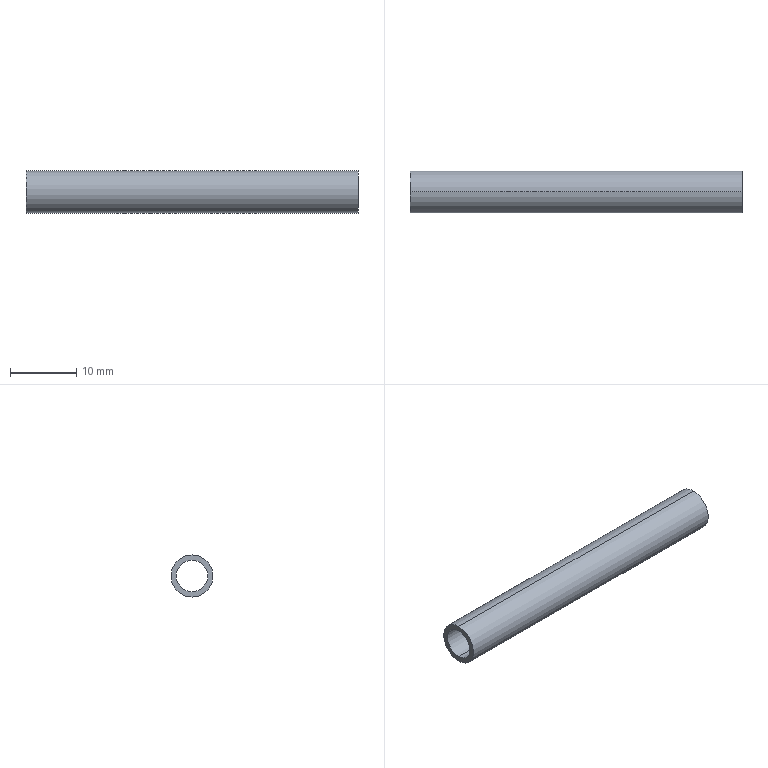Part | STEP file | copper tube 28_default_machined_ | 1 solid | 6 faces | box 50 x 6.35 x 6.35 mm | volume 697.434 mm3 | cylinder 4 | plane 2 | commonest cylinder face diameters 4.75 x2 6.35 x2
STEP:
#1=CARTESIAN_POINT('',(0.,0.,0.));
#2=DIRECTION('',(0.,0.,1.));
#3=DIRECTION('',(1.,0.,0.));
#4=AXIS2_PLACEMENT_3D('',#1,#2,#3);
#5=CARTESIAN_POINT('',(-50.,0.,-3.175));
#6=VERTEX_POINT('',#5);
#7=CARTESIAN_POINT('',(-50.,0.,3.175));
#8=VERTEX_POINT('',#7);
#9=CARTESIAN_POINT('',(-50.,0.,0.));
#10=DIRECTION('',(1.,0.,0.));
#11=DIRECTION('',(0.,0.,-1.));
#12=AXIS2_PLACEMENT_3D('',#9,#10,#11);
#13=CIRCLE('',#12,3.175);
#14=CARTESIAN_POINT('',(-50.,0.,0.));
#15=DIRECTION('',(1.,0.,0.));
#16=DIRECTION('',(0.,0.,-1.));
#17=AXIS2_PLACEMENT_3D('',#14,#15,#16);
#18=CYLINDRICAL_SURFACE('',#17,3.175);
#19=CARTESIAN_POINT('',(0.,0.));
#20=DIRECTION('',(1.,0.));
#21=VECTOR('',#20,1.);
#22=LINE('',#19,#21);
#23=(GEOMETRIC_REPRESENTATION_CONTEXT(2)PARAMETRIC_REPRESENTATION_CONTEXT()REPRESENTATION_CONTEXT('',''));
#24=DEFINITIONAL_REPRESENTATION('',(#22),#23);
#25=PCURVE('',#18,#24);
#26=CARTESIAN_POINT('',(-50.,0.,0.));
#27=DIRECTION('',(-1.,0.,0.));
#28=DIRECTION('',(0.,0.,1.));
#29=AXIS2_PLACEMENT_3D('',#26,#27,#28);
#30=PLANE('',#29);
#31=CARTESIAN_POINT('',(-3.175,0.));
#32=CARTESIAN_POINT('',(-3.175,5.499));
#33=CARTESIAN_POINT('',(1.587,2.75));
#34=CARTESIAN_POINT('',(6.35,0.));
#35=CARTESIAN_POINT('',(1.587,-2.75));
#36=CARTESIAN_POINT('',(-3.175,-5.499));
#37=CARTESIAN_POINT('',(-3.175,0.));
#38=(BOUNDED_CURVE()B_SPLINE_CURVE(2,(#31,#32,#33,#34,#35,#36,#37),.UNSPECIFIED.,.T.,.F.)B_SPLINE_CURVE_WITH_KNOTS((1,2,2,2,2,1),(-2.094,0.,2.094,4.189,6.283,8.378),.UNSPECIFIED.)CURVE()GEOMETRIC_REPRESENTATION_ITEM()RATIONAL_B_SPLINE_CURVE((1.,0.5,1.,0.5,1.,0.5,1.))REPRESENTATION_ITEM(''));
#39=(GEOMETRIC_REPRESENTATION_CONTEXT(2)PARAMETRIC_REPRESENTATION_CONTEXT()REPRESENTATION_CONTEXT('',''));
#40=DEFINITIONAL_REPRESENTATION('',(#38),#39);
#41=PCURVE('',#30,#40);
#42=SURFACE_CURVE('',#13,(#25,#41),.PCURVE_S1.);
#43=EDGE_CURVE('',#6,#8,#42,.T.);
#44=ORIENTED_EDGE('',*,*,#43,.T.);
#45=CARTESIAN_POINT('',(0.,0.,3.175));
#46=VERTEX_POINT('',#45);
#47=CARTESIAN_POINT('',(-50.,0.,3.175));
#48=DIRECTION('',(1.,0.,0.));
#49=VECTOR('',#48,1.);
#50=LINE('',#47,#49);
#51=CARTESIAN_POINT('',(3.142,0.));
#52=DIRECTION('',(0.,1.));
#53=VECTOR('',#52,1.);
#54=LINE('',#51,#53);
#55=(GEOMETRIC_REPRESENTATION_CONTEXT(2)PARAMETRIC_REPRESENTATION_CONTEXT()REPRESENTATION_CONTEXT('',''));
#56=DEFINITIONAL_REPRESENTATION('',(#54),#55);
#57=PCURVE('',#18,#56);
#58=CARTESIAN_POINT('',(-50.,0.,0.));
#59=DIRECTION('',(1.,0.,0.));
#60=DIRECTION('',(0.,0.,-1.));
#61=AXIS2_PLACEMENT_3D('',#58,#59,#60);
#62=CYLINDRICAL_SURFACE('',#61,3.175);
#63=CARTESIAN_POINT('',(3.142,0.));
#64=DIRECTION('',(0.,1.));
#65=VECTOR('',#64,1.);
#66=LINE('',#63,#65);
#67=(GEOMETRIC_REPRESENTATION_CONTEXT(2)PARAMETRIC_REPRESENTATION_CONTEXT()REPRESENTATION_CONTEXT('',''));
#68=DEFINITIONAL_REPRESENTATION('',(#66),#67);
#69=PCURVE('',#62,#68);
#70=SURFACE_CURVE('',#50,(#57,#69),.PCURVE_S1.);
#71=EDGE_CURVE('',#8,#46,#70,.T.);
#72=ORIENTED_EDGE('',*,*,#71,.T.);
#73=CARTESIAN_POINT('',(0.,0.,-3.175));
#74=VERTEX_POINT('',#73);
#75=CARTESIAN_POINT('',(0.,0.,0.));
#76=DIRECTION('',(-1.,0.,0.));
#77=DIRECTION('',(0.,0.,-1.));
#78=AXIS2_PLACEMENT_3D('',#75,#76,#77);
#79=CIRCLE('',#78,3.175);
#80=CARTESIAN_POINT('',(6.283,50.));
#81=DIRECTION('',(-1.,0.));
#82=VECTOR('',#81,1.);
#83=LINE('',#80,#82);
#84=(GEOMETRIC_REPRESENTATION_CONTEXT(2)PARAMETRIC_REPRESENTATION_CONTEXT()REPRESENTATION_CONTEXT('',''));
#85=DEFINITIONAL_REPRESENTATION('',(#83),#84);
#86=PCURVE('',#18,#85);
#87=CARTESIAN_POINT('',(0.,0.,0.));
#88=DIRECTION('',(-1.,0.,0.));
#89=DIRECTION('',(0.,0.,1.));
#90=AXIS2_PLACEMENT_3D('',#87,#88,#89);
#91=PLANE('',#90);
#92=CARTESIAN_POINT('',(0.,0.));
#93=DIRECTION('',(-1.,0.));
#94=AXIS2_PLACEMENT_2D('',#92,#93);
#95=CIRCLE('',#94,3.175);
#96=(GEOMETRIC_REPRESENTATION_CONTEXT(2)PARAMETRIC_REPRESENTATION_CONTEXT()REPRESENTATION_CONTEXT('',''));
#97=DEFINITIONAL_REPRESENTATION('',(#95),#96);
#98=PCURVE('',#91,#97);
#99=SURFACE_CURVE('',#79,(#86,#98),.PCURVE_S1.);
#100=EDGE_CURVE('',#46,#74,#99,.T.);
#101=ORIENTED_EDGE('',*,*,#100,.T.);
#102=CARTESIAN_POINT('',(-50.,0.,-3.175));
#103=DIRECTION('',(1.,0.,0.));
#104=VECTOR('',#103,1.);
#105=LINE('',#102,#104);
#106=CARTESIAN_POINT('',(0.,0.));
#107=DIRECTION('',(0.,1.));
#108=VECTOR('',#107,1.);
#109=LINE('',#106,#108);
#110=(GEOMETRIC_REPRESENTATION_CONTEXT(2)PARAMETRIC_REPRESENTATION_CONTEXT()REPRESENTATION_CONTEXT('',''));
#111=DEFINITIONAL_REPRESENTATION('',(#109),#110);
#112=PCURVE('',#18,#111);
#113=CARTESIAN_POINT('',(6.283,0.));
#114=DIRECTION('',(0.,1.));
#115=VECTOR('',#114,1.);
#116=LINE('',#113,#115);
#117=(GEOMETRIC_REPRESENTATION_CONTEXT(2)PARAMETRIC_REPRESENTATION_CONTEXT()REPRESENTATION_CONTEXT('',''));
#118=DEFINITIONAL_REPRESENTATION('',(#116),#117);
#119=PCURVE('',#62,#118);
#120=SURFACE_CURVE('',#105,(#112,#119),.PCURVE_S1.);
#121=EDGE_CURVE('',#6,#74,#120,.T.);
#122=ORIENTED_EDGE('',*,*,#121,.F.);
#123=EDGE_LOOP('',(#44,#72,#101,#122));
#124=FACE_BOUND('',#123,.T.);
#125=ADVANCED_FACE('',(#124),#18,.T.);
#126=CARTESIAN_POINT('',(-50.,0.,-2.375));
#127=VERTEX_POINT('',#126);
#128=CARTESIAN_POINT('',(0.,0.,-2.375));
#129=VERTEX_POINT('',#128);
#130=CARTESIAN_POINT('',(-50.,0.,-2.375));
#131=DIRECTION('',(1.,0.,0.));
#132=VECTOR('',#131,1.);
#133=LINE('',#130,#132);
#134=CARTESIAN_POINT('',(-50.,0.,0.));
#135=DIRECTION('',(1.,0.,0.));
#136=DIRECTION('',(0.,0.,-1.));
#137=AXIS2_PLACEMENT_3D('',#134,#135,#136);
#138=CYLINDRICAL_SURFACE('',#137,2.375);
#139=CARTESIAN_POINT('',(6.283,0.));
#140=DIRECTION('',(0.,1.));
#141=VECTOR('',#140,1.);
#142=LINE('',#139,#141);
#143=(GEOMETRIC_REPRESENTATION_CONTEXT(2)PARAMETRIC_REPRESENTATION_CONTEXT()REPRESENTATION_CONTEXT('',''));
#144=DEFINITIONAL_REPRESENTATION('',(#142),#143);
#145=PCURVE('',#138,#144);
#146=CARTESIAN_POINT('',(-50.,0.,0.));
#147=DIRECTION('',(1.,0.,0.));
#148=DIRECTION('',(0.,0.,-1.));
#149=AXIS2_PLACEMENT_3D('',#146,#147,#148);
#150=CYLINDRICAL_SURFACE('',#149,2.375);
#151=CARTESIAN_POINT('',(0.,0.));
#152=DIRECTION('',(0.,1.));
#153=VECTOR('',#152,1.);
#154=LINE('',#151,#153);
#155=(GEOMETRIC_REPRESENTATION_CONTEXT(2)PARAMETRIC_REPRESENTATION_CONTEXT()REPRESENTATION_CONTEXT('',''));
#156=DEFINITIONAL_REPRESENTATION('',(#154),#155);
#157=PCURVE('',#150,#156);
#158=SURFACE_CURVE('',#133,(#145,#157),.PCURVE_S1.);
#159=EDGE_CURVE('',#127,#129,#158,.T.);
#160=ORIENTED_EDGE('',*,*,#159,.T.);
#161=CARTESIAN_POINT('',(0.,0.,2.375));
#162=VERTEX_POINT('',#161);
#163=CARTESIAN_POINT('',(0.,0.,0.));
#164=DIRECTION('',(1.,0.,0.));
#165=DIRECTION('',(0.,0.,-1.));
#166=AXIS2_PLACEMENT_3D('',#163,#164,#165);
#167=CIRCLE('',#166,2.375);
#168=CARTESIAN_POINT('',(0.,50.));
#169=DIRECTION('',(1.,0.));
#170=VECTOR('',#169,1.);
#171=LINE('',#168,#170);
#172=(GEOMETRIC_REPRESENTATION_CONTEXT(2)PARAMETRIC_REPRESENTATION_CONTEXT()REPRESENTATION_CONTEXT('',''));
#173=DEFINITIONAL_REPRESENTATION('',(#171),#172);
#174=PCURVE('',#138,#173);
#175=CARTESIAN_POINT('',(-2.375,0.));
#176=CARTESIAN_POINT('',(-2.375,4.114));
#177=CARTESIAN_POINT('',(1.188,2.057));
#178=CARTESIAN_POINT('',(4.75,0.));
#179=CARTESIAN_POINT('',(1.188,-2.057));
#180=CARTESIAN_POINT('',(-2.375,-4.114));
#181=CARTESIAN_POINT('',(-2.375,0.));
#182=(BOUNDED_CURVE()B_SPLINE_CURVE(2,(#175,#176,#177,#178,#179,#180,#181),.UNSPECIFIED.,.T.,.F.)B_SPLINE_CURVE_WITH_KNOTS((1,2,2,2,2,1),(-2.094,0.,2.094,4.189,6.283,8.378),.UNSPECIFIED.)CURVE()GEOMETRIC_REPRESENTATION_ITEM()RATIONAL_B_SPLINE_CURVE((1.,0.5,1.,0.5,1.,0.5,1.))REPRESENTATION_ITEM(''));
#183=(GEOMETRIC_REPRESENTATION_CONTEXT(2)PARAMETRIC_REPRESENTATION_CONTEXT()REPRESENTATION_CONTEXT('',''));
#184=DEFINITIONAL_REPRESENTATION('',(#182),#183);
#185=PCURVE('',#91,#184);
#186=SURFACE_CURVE('',#167,(#174,#185),.PCURVE_S1.);
#187=EDGE_CURVE('',#162,#129,#186,.T.);
#188=ORIENTED_EDGE('',*,*,#187,.F.);
#189=CARTESIAN_POINT('',(-50.,0.,2.375));
#190=VERTEX_POINT('',#189);
#191=CARTESIAN_POINT('',(-50.,0.,2.375));
#192=DIRECTION('',(1.,0.,0.));
#193=VECTOR('',#192,1.);
#194=LINE('',#191,#193);
#195=CARTESIAN_POINT('',(3.142,0.));
#196=DIRECTION('',(0.,1.));
#197=VECTOR('',#196,1.);
#198=LINE('',#195,#197);
#199=(GEOMETRIC_REPRESENTATION_CONTEXT(2)PARAMETRIC_REPRESENTATION_CONTEXT()REPRESENTATION_CONTEXT('',''));
#200=DEFINITIONAL_REPRESENTATION('',(#198),#199);
#201=PCURVE('',#138,#200);
#202=CARTESIAN_POINT('',(3.142,0.));
#203=DIRECTION('',(0.,1.));
#204=VECTOR('',#203,1.);
#205=LINE('',#202,#204);
#206=(GEOMETRIC_REPRESENTATION_CONTEXT(2)PARAMETRIC_REPRESENTATION_CONTEXT()REPRESENTATION_CONTEXT('',''));
#207=DEFINITIONAL_REPRESENTATION('',(#205),#206);
#208=PCURVE('',#150,#207);
#209=SURFACE_CURVE('',#194,(#201,#208),.PCURVE_S1.);
#210=EDGE_CURVE('',#190,#162,#209,.T.);
#211=ORIENTED_EDGE('',*,*,#210,.F.);
#212=CARTESIAN_POINT('',(-50.,0.,0.));
#213=DIRECTION('',(1.,0.,0.));
#214=DIRECTION('',(0.,0.,-1.));
#215=AXIS2_PLACEMENT_3D('',#212,#213,#214);
#216=CIRCLE('',#215,2.375);
#217=CARTESIAN_POINT('',(0.,0.));
#218=DIRECTION('',(1.,0.));
#219=VECTOR('',#218,1.);
#220=LINE('',#217,#219);
#221=(GEOMETRIC_REPRESENTATION_CONTEXT(2)PARAMETRIC_REPRESENTATION_CONTEXT()REPRESENTATION_CONTEXT('',''));
#222=DEFINITIONAL_REPRESENTATION('',(#220),#221);
#223=PCURVE('',#138,#222);
#224=CARTESIAN_POINT('',(-2.375,0.));
#225=CARTESIAN_POINT('',(-2.375,4.114));
#226=CARTESIAN_POINT('',(1.188,2.057));
#227=CARTESIAN_POINT('',(4.75,0.));
#228=CARTESIAN_POINT('',(1.188,-2.057));
#229=CARTESIAN_POINT('',(-2.375,-4.114));
#230=CARTESIAN_POINT('',(-2.375,0.));
#231=(BOUNDED_CURVE()B_SPLINE_CURVE(2,(#224,#225,#226,#227,#228,#229,#230),.UNSPECIFIED.,.T.,.F.)B_SPLINE_CURVE_WITH_KNOTS((1,2,2,2,2,1),(-2.094,0.,2.094,4.189,6.283,8.378),.UNSPECIFIED.)CURVE()GEOMETRIC_REPRESENTATION_ITEM()RATIONAL_B_SPLINE_CURVE((1.,0.5,1.,0.5,1.,0.5,1.))REPRESENTATION_ITEM(''));
#232=(GEOMETRIC_REPRESENTATION_CONTEXT(2)PARAMETRIC_REPRESENTATION_CONTEXT()REPRESENTATION_CONTEXT('',''));
#233=DEFINITIONAL_REPRESENTATION('',(#231),#232);
#234=PCURVE('',#30,#233);
#235=SURFACE_CURVE('',#216,(#223,#234),.PCURVE_S1.);
#236=EDGE_CURVE('',#190,#127,#235,.T.);
#237=ORIENTED_EDGE('',*,*,#236,.T.);
#238=EDGE_LOOP('',(#160,#188,#211,#237));
#239=FACE_BOUND('',#238,.F.);
#240=ADVANCED_FACE('',(#239),#138,.F.);
#241=ORIENTED_EDGE('',*,*,#71,.F.);
#242=CARTESIAN_POINT('',(-50.,0.,0.));
#243=DIRECTION('',(1.,0.,0.));
#244=DIRECTION('',(0.,0.,-1.));
#245=AXIS2_PLACEMENT_3D('',#242,#243,#244);
#246=CIRCLE('',#245,3.175);
#247=CARTESIAN_POINT('',(0.,0.));
#248=DIRECTION('',(1.,0.));
#249=VECTOR('',#248,1.);
#250=LINE('',#247,#249);
#251=(GEOMETRIC_REPRESENTATION_CONTEXT(2)PARAMETRIC_REPRESENTATION_CONTEXT()REPRESENTATION_CONTEXT('',''));
#252=DEFINITIONAL_REPRESENTATION('',(#250),#251);
#253=PCURVE('',#62,#252);
#254=CARTESIAN_POINT('',(-3.175,0.));
#255=CARTESIAN_POINT('',(-3.175,5.499));
#256=CARTESIAN_POINT('',(1.587,2.75));
#257=CARTESIAN_POINT('',(6.35,0.));
#258=CARTESIAN_POINT('',(1.587,-2.75));
#259=CARTESIAN_POINT('',(-3.175,-5.499));
#260=CARTESIAN_POINT('',(-3.175,0.));
#261=(BOUNDED_CURVE()B_SPLINE_CURVE(2,(#254,#255,#256,#257,#258,#259,#260),.UNSPECIFIED.,.T.,.F.)B_SPLINE_CURVE_WITH_KNOTS((1,2,2,2,2,1),(-2.094,0.,2.094,4.189,6.283,8.378),.UNSPECIFIED.)CURVE()GEOMETRIC_REPRESENTATION_ITEM()RATIONAL_B_SPLINE_CURVE((1.,0.5,1.,0.5,1.,0.5,1.))REPRESENTATION_ITEM(''));
#262=(GEOMETRIC_REPRESENTATION_CONTEXT(2)PARAMETRIC_REPRESENTATION_CONTEXT()REPRESENTATION_CONTEXT('',''));
#263=DEFINITIONAL_REPRESENTATION('',(#261),#262);
#264=PCURVE('',#30,#263);
#265=SURFACE_CURVE('',#246,(#253,#264),.PCURVE_S1.);
#266=EDGE_CURVE('',#8,#6,#265,.T.);
#267=ORIENTED_EDGE('',*,*,#266,.T.);
#268=ORIENTED_EDGE('',*,*,#121,.T.);
#269=CARTESIAN_POINT('',(0.,0.,0.));
#270=DIRECTION('',(-1.,0.,0.));
#271=DIRECTION('',(0.,0.,-1.));
#272=AXIS2_PLACEMENT_3D('',#269,#270,#271);
#273=CIRCLE('',#272,3.175);
#274=CARTESIAN_POINT('',(6.283,50.));
#275=DIRECTION('',(-1.,0.));
#276=VECTOR('',#275,1.);
#277=LINE('',#274,#276);
#278=(GEOMETRIC_REPRESENTATION_CONTEXT(2)PARAMETRIC_REPRESENTATION_CONTEXT()REPRESENTATION_CONTEXT('',''));
#279=DEFINITIONAL_REPRESENTATION('',(#277),#278);
#280=PCURVE('',#62,#279);
#281=CARTESIAN_POINT('',(0.,0.));
#282=DIRECTION('',(-1.,0.));
#283=AXIS2_PLACEMENT_2D('',#281,#282);
#284=CIRCLE('',#283,3.175);
#285=(GEOMETRIC_REPRESENTATION_CONTEXT(2)PARAMETRIC_REPRESENTATION_CONTEXT()REPRESENTATION_CONTEXT('',''));
#286=DEFINITIONAL_REPRESENTATION('',(#284),#285);
#287=PCURVE('',#91,#286);
#288=SURFACE_CURVE('',#273,(#280,#287),.PCURVE_S1.);
#289=EDGE_CURVE('',#74,#46,#288,.T.);
#290=ORIENTED_EDGE('',*,*,#289,.T.);
#291=EDGE_LOOP('',(#241,#267,#268,#290));
#292=FACE_BOUND('',#291,.T.);
#293=ADVANCED_FACE('',(#292),#62,.T.);
#294=ORIENTED_EDGE('',*,*,#289,.F.);
#295=ORIENTED_EDGE('',*,*,#100,.F.);
#296=EDGE_LOOP('',(#294,#295));
#297=FACE_BOUND('',#296,.T.);
#298=CARTESIAN_POINT('',(0.,0.,0.));
#299=DIRECTION('',(1.,0.,0.));
#300=DIRECTION('',(0.,0.,-1.));
#301=AXIS2_PLACEMENT_3D('',#298,#299,#300);
#302=CIRCLE('',#301,2.375);
#303=CARTESIAN_POINT('',(-2.375,0.));
#304=CARTESIAN_POINT('',(-2.375,4.114));
#305=CARTESIAN_POINT('',(1.188,2.057));
#306=CARTESIAN_POINT('',(4.75,0.));
#307=CARTESIAN_POINT('',(1.188,-2.057));
#308=CARTESIAN_POINT('',(-2.375,-4.114));
#309=CARTESIAN_POINT('',(-2.375,0.));
#310=(BOUNDED_CURVE()B_SPLINE_CURVE(2,(#303,#304,#305,#306,#307,#308,#309),.UNSPECIFIED.,.T.,.F.)B_SPLINE_CURVE_WITH_KNOTS((1,2,2,2,2,1),(-2.094,0.,2.094,4.189,6.283,8.378),.UNSPECIFIED.)CURVE()GEOMETRIC_REPRESENTATION_ITEM()RATIONAL_B_SPLINE_CURVE((1.,0.5,1.,0.5,1.,0.5,1.))REPRESENTATION_ITEM(''));
#311=(GEOMETRIC_REPRESENTATION_CONTEXT(2)PARAMETRIC_REPRESENTATION_CONTEXT()REPRESENTATION_CONTEXT('',''));
#312=DEFINITIONAL_REPRESENTATION('',(#310),#311);
#313=PCURVE('',#91,#312);
#314=CARTESIAN_POINT('',(0.,50.));
#315=DIRECTION('',(1.,0.));
#316=VECTOR('',#315,1.);
#317=LINE('',#314,#316);
#318=(GEOMETRIC_REPRESENTATION_CONTEXT(2)PARAMETRIC_REPRESENTATION_CONTEXT()REPRESENTATION_CONTEXT('',''));
#319=DEFINITIONAL_REPRESENTATION('',(#317),#318);
#320=PCURVE('',#150,#319);
#321=SURFACE_CURVE('',#302,(#313,#320),.PCURVE_S1.);
#322=EDGE_CURVE('',#129,#162,#321,.T.);
#323=ORIENTED_EDGE('',*,*,#322,.F.);
#324=ORIENTED_EDGE('',*,*,#187,.F.);
#325=EDGE_LOOP('',(#323,#324));
#326=FACE_BOUND('',#325,.T.);
#327=ADVANCED_FACE('',(#297,#326),#91,.F.);
#328=ORIENTED_EDGE('',*,*,#43,.F.);
#329=ORIENTED_EDGE('',*,*,#266,.F.);
#330=EDGE_LOOP('',(#328,#329));
#331=FACE_BOUND('',#330,.T.);
#332=CARTESIAN_POINT('',(-50.,0.,0.));
#333=DIRECTION('',(1.,0.,0.));
#334=DIRECTION('',(0.,0.,-1.));
#335=AXIS2_PLACEMENT_3D('',#332,#333,#334);
#336=CIRCLE('',#335,2.375);
#337=CARTESIAN_POINT('',(-2.375,0.));
#338=CARTESIAN_POINT('',(-2.375,4.114));
#339=CARTESIAN_POINT('',(1.188,2.057));
#340=CARTESIAN_POINT('',(4.75,0.));
#341=CARTESIAN_POINT('',(1.188,-2.057));
#342=CARTESIAN_POINT('',(-2.375,-4.114));
#343=CARTESIAN_POINT('',(-2.375,0.));
#344=(BOUNDED_CURVE()B_SPLINE_CURVE(2,(#337,#338,#339,#340,#341,#342,#343),.UNSPECIFIED.,.T.,.F.)B_SPLINE_CURVE_WITH_KNOTS((1,2,2,2,2,1),(-2.094,0.,2.094,4.189,6.283,8.378),.UNSPECIFIED.)CURVE()GEOMETRIC_REPRESENTATION_ITEM()RATIONAL_B_SPLINE_CURVE((1.,0.5,1.,0.5,1.,0.5,1.))REPRESENTATION_ITEM(''));
#345=(GEOMETRIC_REPRESENTATION_CONTEXT(2)PARAMETRIC_REPRESENTATION_CONTEXT()REPRESENTATION_CONTEXT('',''));
#346=DEFINITIONAL_REPRESENTATION('',(#344),#345);
#347=PCURVE('',#30,#346);
#348=CARTESIAN_POINT('',(0.,0.));
#349=DIRECTION('',(1.,0.));
#350=VECTOR('',#349,1.);
#351=LINE('',#348,#350);
#352=(GEOMETRIC_REPRESENTATION_CONTEXT(2)PARAMETRIC_REPRESENTATION_CONTEXT()REPRESENTATION_CONTEXT('',''));
#353=DEFINITIONAL_REPRESENTATION('',(#351),#352);
#354=PCURVE('',#150,#353);
#355=SURFACE_CURVE('',#336,(#347,#354),.PCURVE_S1.);
#356=EDGE_CURVE('',#127,#190,#355,.T.);
#357=ORIENTED_EDGE('',*,*,#356,.T.);
#358=ORIENTED_EDGE('',*,*,#236,.T.);
#359=EDGE_LOOP('',(#357,#358));
#360=FACE_BOUND('',#359,.T.);
#361=ADVANCED_FACE('',(#331,#360),#30,.T.);
#362=ORIENTED_EDGE('',*,*,#322,.F.);
#363=ORIENTED_EDGE('',*,*,#159,.F.);
#364=ORIENTED_EDGE('',*,*,#356,.T.);
#365=ORIENTED_EDGE('',*,*,#210,.T.);
#366=EDGE_LOOP('',(#362,#363,#364,#365));
#367=FACE_BOUND('',#366,.F.);
#368=ADVANCED_FACE('',(#367),#150,.F.);
#369=CLOSED_SHELL('',(#125,#240,#293,#327,#361,#368));
#370=MANIFOLD_SOLID_BREP('',#369);
#371=(LENGTH_UNIT()NAMED_UNIT(*)SI_UNIT(.MILLI.,.METRE.));
#372=UNCERTAINTY_MEASURE_WITH_UNIT(LENGTH_MEASURE(0.0000001),#371,'','');
#373=(NAMED_UNIT(*)PLANE_ANGLE_UNIT()SI_UNIT($,.RADIAN.));
#374=(NAMED_UNIT(*)SI_UNIT($,.STERADIAN.)SOLID_ANGLE_UNIT());
#375=(GEOMETRIC_REPRESENTATION_CONTEXT(3)GLOBAL_UNCERTAINTY_ASSIGNED_CONTEXT((#372))GLOBAL_UNIT_ASSIGNED_CONTEXT((#371,#373,#374))REPRESENTATION_CONTEXT('',''));
#376=ADVANCED_BREP_SHAPE_REPRESENTATION('',(#4,#370),#375);